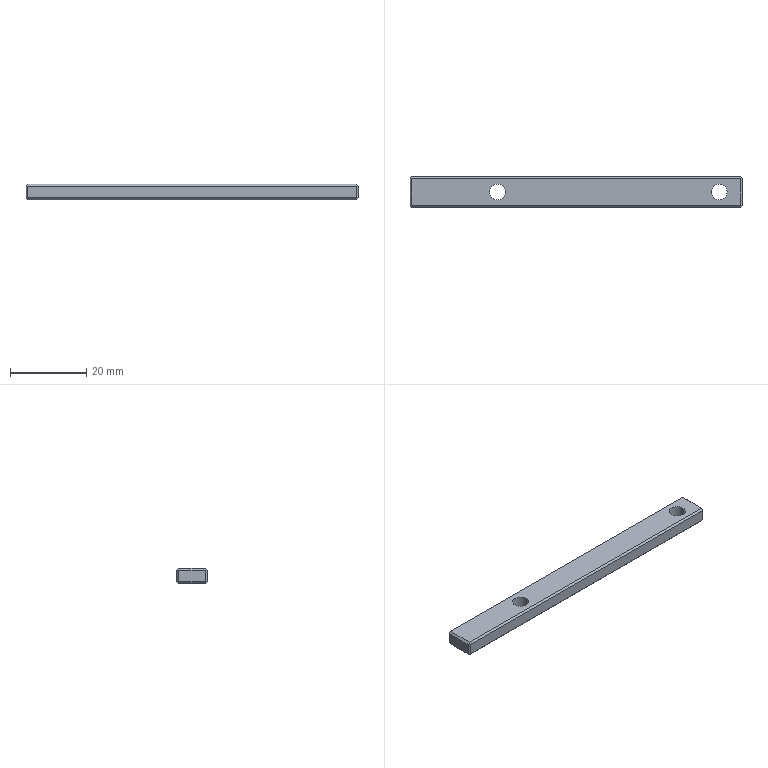Part | Creo | features DATUM PLANE 3, CHAMFER 1, COORDINATE SYSTEM 1, CURVE 1, PROTRUSION 1 | 1 solid | 22 faces | box 87 x 8 x 4 mm | volume 2624 mm3 | plane 18 | cylinder 4 | commonest cylinder face diameters 4.2 x4
STEP:
#1=CARTESIAN_POINT('',(0.,0.,0.));
#2=DIRECTION('',(0.,0.,1.));
#3=DIRECTION('',(1.,0.,0.));
#4=AXIS2_PLACEMENT_3D('',#1,#2,#3);
#5=CARTESIAN_POINT('',(43.,3.5,0.));
#6=VERTEX_POINT('',#5);
#7=CARTESIAN_POINT('',(43.,-3.5,0.));
#8=VERTEX_POINT('',#7);
#9=CARTESIAN_POINT('',(43.,3.5,0.));
#10=DIRECTION('',(0.,-1.,0.));
#11=VECTOR('',#10,7.);
#12=LINE('',#9,#11);
#13=EDGE_CURVE('',#6,#8,#12,.T.);
#14=ORIENTED_EDGE('',*,*,#13,.F.);
#15=CARTESIAN_POINT('',(-43.,3.5,0.));
#16=VERTEX_POINT('',#15);
#17=CARTESIAN_POINT('',(-43.,3.5,0.));
#18=DIRECTION('',(1.,0.,0.));
#19=VECTOR('',#18,86.);
#20=LINE('',#17,#19);
#21=EDGE_CURVE('',#16,#6,#20,.T.);
#22=ORIENTED_EDGE('',*,*,#21,.F.);
#23=CARTESIAN_POINT('',(-43.,-3.5,0.));
#24=VERTEX_POINT('',#23);
#25=CARTESIAN_POINT('',(-43.,-3.5,0.));
#26=DIRECTION('',(0.,1.,0.));
#27=VECTOR('',#26,7.);
#28=LINE('',#25,#27);
#29=EDGE_CURVE('',#24,#16,#28,.T.);
#30=ORIENTED_EDGE('',*,*,#29,.F.);
#31=CARTESIAN_POINT('',(43.,-3.5,0.));
#32=DIRECTION('',(-1.,0.,0.));
#33=VECTOR('',#32,86.);
#34=LINE('',#31,#33);
#35=EDGE_CURVE('',#8,#24,#34,.T.);
#36=ORIENTED_EDGE('',*,*,#35,.F.);
#37=EDGE_LOOP('',(#14,#22,#30,#36));
#38=FACE_OUTER_BOUND('',#37,.F.);
#39=CARTESIAN_POINT('',(-18.4,0.,0.));
#40=VERTEX_POINT('',#39);
#41=CARTESIAN_POINT('',(-22.6,0.,0.));
#42=VERTEX_POINT('',#41);
#43=CARTESIAN_POINT('',(-20.5,0.,0.));
#44=DIRECTION('',(0.,0.,-1.));
#45=DIRECTION('',(1.,0.,0.));
#46=AXIS2_PLACEMENT_3D('',#43,#44,#45);
#47=CIRCLE('',#46,2.1);
#48=EDGE_CURVE('',#40,#42,#47,.T.);
#49=ORIENTED_EDGE('',*,*,#48,.T.);
#50=CARTESIAN_POINT('',(-20.5,0.,0.));
#51=DIRECTION('',(0.,0.,-1.));
#52=DIRECTION('',(-1.,0.,0.));
#53=AXIS2_PLACEMENT_3D('',#50,#51,#52);
#54=CIRCLE('',#53,2.1);
#55=EDGE_CURVE('',#42,#40,#54,.T.);
#56=ORIENTED_EDGE('',*,*,#55,.T.);
#57=EDGE_LOOP('',(#49,#56));
#58=FACE_BOUND('',#57,.F.);
#59=CARTESIAN_POINT('',(39.6,0.,0.));
#60=VERTEX_POINT('',#59);
#61=CARTESIAN_POINT('',(35.4,0.,0.));
#62=VERTEX_POINT('',#61);
#63=CARTESIAN_POINT('',(37.5,0.,0.));
#64=DIRECTION('',(0.,0.,-1.));
#65=DIRECTION('',(1.,0.,0.));
#66=AXIS2_PLACEMENT_3D('',#63,#64,#65);
#67=CIRCLE('',#66,2.1);
#68=EDGE_CURVE('',#60,#62,#67,.T.);
#69=ORIENTED_EDGE('',*,*,#68,.T.);
#70=CARTESIAN_POINT('',(37.5,0.,0.));
#71=DIRECTION('',(0.,0.,-1.));
#72=DIRECTION('',(-1.,0.,0.));
#73=AXIS2_PLACEMENT_3D('',#70,#71,#72);
#74=CIRCLE('',#73,2.1);
#75=EDGE_CURVE('',#62,#60,#74,.T.);
#76=ORIENTED_EDGE('',*,*,#75,.T.);
#77=EDGE_LOOP('',(#69,#76));
#78=FACE_BOUND('',#77,.F.);
#79=CARTESIAN_POINT('',(0.,0.,0.));
#80=DIRECTION('',(0.,0.,1.));
#81=DIRECTION('',(1.,0.,0.));
#82=AXIS2_PLACEMENT_3D('',#79,#80,#81);
#83=PLANE('',#82);
#84=ADVANCED_FACE('',(#38,#58,#78),#83,.F.);
#85=ORIENTED_EDGE('',*,*,#68,.F.);
#86=CARTESIAN_POINT('',(39.6,0.,4.));
#87=VERTEX_POINT('',#86);
#88=CARTESIAN_POINT('',(39.6,0.,0.));
#89=DIRECTION('',(0.,0.,1.));
#90=VECTOR('',#89,4.);
#91=LINE('',#88,#90);
#92=EDGE_CURVE('',#60,#87,#91,.T.);
#93=ORIENTED_EDGE('',*,*,#92,.T.);
#94=CARTESIAN_POINT('',(35.4,0.,4.));
#95=VERTEX_POINT('',#94);
#96=CARTESIAN_POINT('',(37.5,0.,4.));
#97=DIRECTION('',(0.,0.,-1.));
#98=DIRECTION('',(1.,0.,0.));
#99=AXIS2_PLACEMENT_3D('',#96,#97,#98);
#100=CIRCLE('',#99,2.1);
#101=EDGE_CURVE('',#87,#95,#100,.T.);
#102=ORIENTED_EDGE('',*,*,#101,.T.);
#103=CARTESIAN_POINT('',(35.4,0.,0.));
#104=DIRECTION('',(0.,0.,1.));
#105=VECTOR('',#104,4.);
#106=LINE('',#103,#105);
#107=EDGE_CURVE('',#62,#95,#106,.T.);
#108=ORIENTED_EDGE('',*,*,#107,.F.);
#109=EDGE_LOOP('',(#85,#93,#102,#108));
#110=FACE_OUTER_BOUND('',#109,.F.);
#111=CARTESIAN_POINT('',(37.5,0.,0.));
#112=DIRECTION('',(0.,0.,1.));
#113=DIRECTION('',(1.,0.,0.));
#114=AXIS2_PLACEMENT_3D('',#111,#112,#113);
#115=CYLINDRICAL_SURFACE('',#114,2.1);
#116=ADVANCED_FACE('',(#110),#115,.F.);
#117=ORIENTED_EDGE('',*,*,#75,.F.);
#118=ORIENTED_EDGE('',*,*,#107,.T.);
#119=CARTESIAN_POINT('',(37.5,0.,4.));
#120=DIRECTION('',(0.,0.,-1.));
#121=DIRECTION('',(-1.,0.,0.));
#122=AXIS2_PLACEMENT_3D('',#119,#120,#121);
#123=CIRCLE('',#122,2.1);
#124=EDGE_CURVE('',#95,#87,#123,.T.);
#125=ORIENTED_EDGE('',*,*,#124,.T.);
#126=ORIENTED_EDGE('',*,*,#92,.F.);
#127=EDGE_LOOP('',(#117,#118,#125,#126));
#128=FACE_OUTER_BOUND('',#127,.F.);
#129=CARTESIAN_POINT('',(37.5,0.,0.));
#130=DIRECTION('',(0.,0.,1.));
#131=DIRECTION('',(1.,0.,0.));
#132=AXIS2_PLACEMENT_3D('',#129,#130,#131);
#133=CYLINDRICAL_SURFACE('',#132,2.1);
#134=ADVANCED_FACE('',(#128),#133,.F.);
#135=CARTESIAN_POINT('',(43.,-3.5,4.));
#136=VERTEX_POINT('',#135);
#137=CARTESIAN_POINT('',(43.,3.5,4.));
#138=VERTEX_POINT('',#137);
#139=CARTESIAN_POINT('',(43.,-3.5,4.));
#140=DIRECTION('',(0.,1.,0.));
#141=VECTOR('',#140,7.);
#142=LINE('',#139,#141);
#143=EDGE_CURVE('',#136,#138,#142,.T.);
#144=ORIENTED_EDGE('',*,*,#143,.F.);
#145=CARTESIAN_POINT('',(-43.,-3.5,4.));
#146=VERTEX_POINT('',#145);
#147=CARTESIAN_POINT('',(-43.,-3.5,4.));
#148=DIRECTION('',(1.,0.,0.));
#149=VECTOR('',#148,86.);
#150=LINE('',#147,#149);
#151=EDGE_CURVE('',#146,#136,#150,.T.);
#152=ORIENTED_EDGE('',*,*,#151,.F.);
#153=CARTESIAN_POINT('',(-43.,3.5,4.));
#154=VERTEX_POINT('',#153);
#155=CARTESIAN_POINT('',(-43.,3.5,4.));
#156=DIRECTION('',(0.,-1.,0.));
#157=VECTOR('',#156,7.);
#158=LINE('',#155,#157);
#159=EDGE_CURVE('',#154,#146,#158,.T.);
#160=ORIENTED_EDGE('',*,*,#159,.F.);
#161=CARTESIAN_POINT('',(43.,3.5,4.));
#162=DIRECTION('',(-1.,0.,0.));
#163=VECTOR('',#162,86.);
#164=LINE('',#161,#163);
#165=EDGE_CURVE('',#138,#154,#164,.T.);
#166=ORIENTED_EDGE('',*,*,#165,.F.);
#167=EDGE_LOOP('',(#144,#152,#160,#166));
#168=FACE_OUTER_BOUND('',#167,.F.);
#169=CARTESIAN_POINT('',(-18.4,0.,4.));
#170=VERTEX_POINT('',#169);
#171=CARTESIAN_POINT('',(-22.6,0.,4.));
#172=VERTEX_POINT('',#171);
#173=CARTESIAN_POINT('',(-20.5,0.,4.));
#174=DIRECTION('',(0.,0.,-1.));
#175=DIRECTION('',(1.,0.,0.));
#176=AXIS2_PLACEMENT_3D('',#173,#174,#175);
#177=CIRCLE('',#176,2.1);
#178=EDGE_CURVE('',#170,#172,#177,.T.);
#179=ORIENTED_EDGE('',*,*,#178,.F.);
#180=CARTESIAN_POINT('',(-20.5,0.,4.));
#181=DIRECTION('',(0.,0.,-1.));
#182=DIRECTION('',(-1.,0.,0.));
#183=AXIS2_PLACEMENT_3D('',#180,#181,#182);
#184=CIRCLE('',#183,2.1);
#185=EDGE_CURVE('',#172,#170,#184,.T.);
#186=ORIENTED_EDGE('',*,*,#185,.F.);
#187=EDGE_LOOP('',(#179,#186));
#188=FACE_BOUND('',#187,.F.);
#189=ORIENTED_EDGE('',*,*,#101,.F.);
#190=ORIENTED_EDGE('',*,*,#124,.F.);
#191=EDGE_LOOP('',(#189,#190));
#192=FACE_BOUND('',#191,.F.);
#193=CARTESIAN_POINT('',(0.,0.,4.));
#194=DIRECTION('',(0.,0.,1.));
#195=DIRECTION('',(1.,0.,0.));
#196=AXIS2_PLACEMENT_3D('',#193,#194,#195);
#197=PLANE('',#196);
#198=ADVANCED_FACE('',(#168,#188,#192),#197,.T.);
#199=ORIENTED_EDGE('',*,*,#48,.F.);
#200=CARTESIAN_POINT('',(-18.4,0.,0.));
#201=DIRECTION('',(0.,0.,1.));
#202=VECTOR('',#201,4.);
#203=LINE('',#200,#202);
#204=EDGE_CURVE('',#40,#170,#203,.T.);
#205=ORIENTED_EDGE('',*,*,#204,.T.);
#206=ORIENTED_EDGE('',*,*,#178,.T.);
#207=CARTESIAN_POINT('',(-22.6,0.,0.));
#208=DIRECTION('',(0.,0.,1.));
#209=VECTOR('',#208,4.);
#210=LINE('',#207,#209);
#211=EDGE_CURVE('',#42,#172,#210,.T.);
#212=ORIENTED_EDGE('',*,*,#211,.F.);
#213=EDGE_LOOP('',(#199,#205,#206,#212));
#214=FACE_OUTER_BOUND('',#213,.F.);
#215=CARTESIAN_POINT('',(-20.5,0.,0.));
#216=DIRECTION('',(0.,0.,1.));
#217=DIRECTION('',(1.,0.,0.));
#218=AXIS2_PLACEMENT_3D('',#215,#216,#217);
#219=CYLINDRICAL_SURFACE('',#218,2.1);
#220=ADVANCED_FACE('',(#214),#219,.F.);
#221=ORIENTED_EDGE('',*,*,#55,.F.);
#222=ORIENTED_EDGE('',*,*,#211,.T.);
#223=ORIENTED_EDGE('',*,*,#185,.T.);
#224=ORIENTED_EDGE('',*,*,#204,.F.);
#225=EDGE_LOOP('',(#221,#222,#223,#224));
#226=FACE_OUTER_BOUND('',#225,.F.);
#227=CARTESIAN_POINT('',(-20.5,0.,0.));
#228=DIRECTION('',(0.,0.,1.));
#229=DIRECTION('',(1.,0.,0.));
#230=AXIS2_PLACEMENT_3D('',#227,#228,#229);
#231=CYLINDRICAL_SURFACE('',#230,2.1);
#232=ADVANCED_FACE('',(#226),#231,.F.);
#233=CARTESIAN_POINT('',(43.5,-3.5,3.5));
#234=VERTEX_POINT('',#233);
#235=CARTESIAN_POINT('',(43.5,3.5,3.5));
#236=VERTEX_POINT('',#235);
#237=CARTESIAN_POINT('',(43.5,-3.5,3.5));
#238=DIRECTION('',(0.,1.,0.));
#239=VECTOR('',#238,7.);
#240=LINE('',#237,#239);
#241=EDGE_CURVE('',#234,#236,#240,.T.);
#242=ORIENTED_EDGE('',*,*,#241,.F.);
#243=CARTESIAN_POINT('',(43.25,-3.75,3.75));
#244=VERTEX_POINT('',#243);
#245=CARTESIAN_POINT('',(43.5,-3.5,3.5));
#246=DIRECTION('',(-0.5774,-0.5774,0.5774));
#247=VECTOR('',#246,0.433);
#248=LINE('',#245,#247);
#249=EDGE_CURVE('',#234,#244,#248,.T.);
#250=ORIENTED_EDGE('',*,*,#249,.T.);
#251=CARTESIAN_POINT('',(43.25,-3.75,3.75));
#252=DIRECTION('',(-0.5774,0.5774,0.5774));
#253=VECTOR('',#252,0.433);
#254=LINE('',#251,#253);
#255=EDGE_CURVE('',#244,#136,#254,.T.);
#256=ORIENTED_EDGE('',*,*,#255,.T.);
#257=ORIENTED_EDGE('',*,*,#143,.T.);
#258=CARTESIAN_POINT('',(43.25,3.75,3.75));
#259=VERTEX_POINT('',#258);
#260=CARTESIAN_POINT('',(43.,3.5,4.));
#261=DIRECTION('',(0.5774,0.5774,-0.5774));
#262=VECTOR('',#261,0.433);
#263=LINE('',#260,#262);
#264=EDGE_CURVE('',#138,#259,#263,.T.);
#265=ORIENTED_EDGE('',*,*,#264,.T.);
#266=CARTESIAN_POINT('',(43.25,3.75,3.75));
#267=DIRECTION('',(0.5774,-0.5774,-0.5774));
#268=VECTOR('',#267,0.433);
#269=LINE('',#266,#268);
#270=EDGE_CURVE('',#259,#236,#269,.T.);
#271=ORIENTED_EDGE('',*,*,#270,.T.);
#272=EDGE_LOOP('',(#242,#250,#256,#257,#265,#271));
#273=FACE_OUTER_BOUND('',#272,.F.);
#274=CARTESIAN_POINT('',(43.25,0.,3.75));
#275=DIRECTION('',(0.7071,0.,0.7071));
#276=DIRECTION('',(0.7071,0.,-0.7071));
#277=AXIS2_PLACEMENT_3D('',#274,#275,#276);
#278=PLANE('',#277);
#279=ADVANCED_FACE('',(#273),#278,.T.);
#280=CARTESIAN_POINT('',(43.5,3.5,0.5));
#281=VERTEX_POINT('',#280);
#282=CARTESIAN_POINT('',(43.5,-3.5,0.5));
#283=VERTEX_POINT('',#282);
#284=CARTESIAN_POINT('',(43.5,3.5,0.5));
#285=DIRECTION('',(0.,-1.,0.));
#286=VECTOR('',#285,7.);
#287=LINE('',#284,#286);
#288=EDGE_CURVE('',#281,#283,#287,.T.);
#289=ORIENTED_EDGE('',*,*,#288,.T.);
#290=CARTESIAN_POINT('',(43.5,-3.5,3.5));
#291=DIRECTION('',(0.,0.,-1.));
#292=VECTOR('',#291,3.);
#293=LINE('',#290,#292);
#294=EDGE_CURVE('',#234,#283,#293,.T.);
#295=ORIENTED_EDGE('',*,*,#294,.F.);
#296=ORIENTED_EDGE('',*,*,#241,.T.);
#297=CARTESIAN_POINT('',(43.5,3.5,3.5));
#298=DIRECTION('',(0.,0.,-1.));
#299=VECTOR('',#298,3.);
#300=LINE('',#297,#299);
#301=EDGE_CURVE('',#236,#281,#300,.T.);
#302=ORIENTED_EDGE('',*,*,#301,.T.);
#303=EDGE_LOOP('',(#289,#295,#296,#302));
#304=FACE_OUTER_BOUND('',#303,.F.);
#305=CARTESIAN_POINT('',(43.5,-4.,0.));
#306=DIRECTION('',(1.,0.,0.));
#307=DIRECTION('',(0.,1.,0.));
#308=AXIS2_PLACEMENT_3D('',#305,#306,#307);
#309=PLANE('',#308);
#310=ADVANCED_FACE('',(#304),#309,.T.);
#311=ORIENTED_EDGE('',*,*,#288,.F.);
#312=CARTESIAN_POINT('',(43.25,3.75,0.25));
#313=VERTEX_POINT('',#312);
#314=CARTESIAN_POINT('',(43.5,3.5,0.5));
#315=DIRECTION('',(-0.5774,0.5774,-0.5774));
#316=VECTOR('',#315,0.433);
#317=LINE('',#314,#316);
#318=EDGE_CURVE('',#281,#313,#317,.T.);
#319=ORIENTED_EDGE('',*,*,#318,.T.);
#320=CARTESIAN_POINT('',(43.25,3.75,0.25));
#321=DIRECTION('',(-0.5774,-0.5774,-0.5774));
#322=VECTOR('',#321,0.433);
#323=LINE('',#320,#322);
#324=EDGE_CURVE('',#313,#6,#323,.T.);
#325=ORIENTED_EDGE('',*,*,#324,.T.);
#326=ORIENTED_EDGE('',*,*,#13,.T.);
#327=CARTESIAN_POINT('',(43.25,-3.75,0.25));
#328=VERTEX_POINT('',#327);
#329=CARTESIAN_POINT('',(43.,-3.5,0.));
#330=DIRECTION('',(0.5774,-0.5774,0.5774));
#331=VECTOR('',#330,0.433);
#332=LINE('',#329,#331);
#333=EDGE_CURVE('',#8,#328,#332,.T.);
#334=ORIENTED_EDGE('',*,*,#333,.T.);
#335=CARTESIAN_POINT('',(43.25,-3.75,0.25));
#336=DIRECTION('',(0.5774,0.5774,0.5774));
#337=VECTOR('',#336,0.433);
#338=LINE('',#335,#337);
#339=EDGE_CURVE('',#328,#283,#338,.T.);
#340=ORIENTED_EDGE('',*,*,#339,.T.);
#341=EDGE_LOOP('',(#311,#319,#325,#326,#334,#340));
#342=FACE_OUTER_BOUND('',#341,.F.);
#343=CARTESIAN_POINT('',(43.25,0.,0.25));
#344=DIRECTION('',(0.7071,0.,-0.7071));
#345=DIRECTION('',(0.7071,0.,0.7071));
#346=AXIS2_PLACEMENT_3D('',#343,#344,#345);
#347=PLANE('',#346);
#348=ADVANCED_FACE('',(#342),#347,.T.);
#349=CARTESIAN_POINT('',(43.,4.,3.5));
#350=VERTEX_POINT('',#349);
#351=CARTESIAN_POINT('',(43.,4.,0.5));
#352=VERTEX_POINT('',#351);
#353=CARTESIAN_POINT('',(43.,4.,3.5));
#354=DIRECTION('',(0.,0.,-1.));
#355=VECTOR('',#354,3.);
#356=LINE('',#353,#355);
#357=EDGE_CURVE('',#350,#352,#356,.T.);
#358=ORIENTED_EDGE('',*,*,#357,.T.);
#359=CARTESIAN_POINT('',(43.,4.,0.5));
#360=DIRECTION('',(0.5774,-0.5774,-0.5774));
#361=VECTOR('',#360,0.433);
#362=LINE('',#359,#361);
#363=EDGE_CURVE('',#352,#313,#362,.T.);
#364=ORIENTED_EDGE('',*,*,#363,.T.);
#365=ORIENTED_EDGE('',*,*,#318,.F.);
#366=ORIENTED_EDGE('',*,*,#301,.F.);
#367=ORIENTED_EDGE('',*,*,#270,.F.);
#368=CARTESIAN_POINT('',(43.,4.,3.5));
#369=DIRECTION('',(0.5774,-0.5774,0.5774));
#370=VECTOR('',#369,0.433);
#371=LINE('',#368,#370);
#372=EDGE_CURVE('',#350,#259,#371,.T.);
#373=ORIENTED_EDGE('',*,*,#372,.F.);
#374=EDGE_LOOP('',(#358,#364,#365,#366,#367,#373));
#375=FACE_OUTER_BOUND('',#374,.F.);
#376=CARTESIAN_POINT('',(43.25,3.75,2.));
#377=DIRECTION('',(0.7071,0.7071,0.));
#378=DIRECTION('',(0.7071,-0.7071,0.));
#379=AXIS2_PLACEMENT_3D('',#376,#377,#378);
#380=PLANE('',#379);
#381=ADVANCED_FACE('',(#375),#380,.T.);
#382=CARTESIAN_POINT('',(-43.,4.,3.5));
#383=VERTEX_POINT('',#382);
#384=CARTESIAN_POINT('',(43.,4.,3.5));
#385=DIRECTION('',(-1.,0.,0.));
#386=VECTOR('',#385,86.);
#387=LINE('',#384,#386);
#388=EDGE_CURVE('',#350,#383,#387,.T.);
#389=ORIENTED_EDGE('',*,*,#388,.T.);
#390=CARTESIAN_POINT('',(-43.,4.,0.5));
#391=VERTEX_POINT('',#390);
#392=CARTESIAN_POINT('',(-43.,4.,3.5));
#393=DIRECTION('',(0.,0.,-1.));
#394=VECTOR('',#393,3.);
#395=LINE('',#392,#394);
#396=EDGE_CURVE('',#383,#391,#395,.T.);
#397=ORIENTED_EDGE('',*,*,#396,.T.);
#398=CARTESIAN_POINT('',(-43.,4.,0.5));
#399=DIRECTION('',(1.,0.,0.));
#400=VECTOR('',#399,86.);
#401=LINE('',#398,#400);
#402=EDGE_CURVE('',#391,#352,#401,.T.);
#403=ORIENTED_EDGE('',*,*,#402,.T.);
#404=ORIENTED_EDGE('',*,*,#357,.F.);
#405=EDGE_LOOP('',(#389,#397,#403,#404));
#406=FACE_OUTER_BOUND('',#405,.F.);
#407=CARTESIAN_POINT('',(43.5,4.,0.));
#408=DIRECTION('',(0.,1.,0.));
#409=DIRECTION('',(-1.,0.,0.));
#410=AXIS2_PLACEMENT_3D('',#407,#408,#409);
#411=PLANE('',#410);
#412=ADVANCED_FACE('',(#406),#411,.T.);
#413=ORIENTED_EDGE('',*,*,#388,.F.);
#414=ORIENTED_EDGE('',*,*,#372,.T.);
#415=ORIENTED_EDGE('',*,*,#264,.F.);
#416=ORIENTED_EDGE('',*,*,#165,.T.);
#417=CARTESIAN_POINT('',(-43.25,3.75,3.75));
#418=VERTEX_POINT('',#417);
#419=CARTESIAN_POINT('',(-43.,3.5,4.));
#420=DIRECTION('',(-0.5774,0.5774,-0.5774));
#421=VECTOR('',#420,0.433);
#422=LINE('',#419,#421);
#423=EDGE_CURVE('',#154,#418,#422,.T.);
#424=ORIENTED_EDGE('',*,*,#423,.T.);
#425=CARTESIAN_POINT('',(-43.25,3.75,3.75));
#426=DIRECTION('',(0.5774,0.5774,-0.5774));
#427=VECTOR('',#426,0.433);
#428=LINE('',#425,#427);
#429=EDGE_CURVE('',#418,#383,#428,.T.);
#430=ORIENTED_EDGE('',*,*,#429,.T.);
#431=EDGE_LOOP('',(#413,#414,#415,#416,#424,#430));
#432=FACE_OUTER_BOUND('',#431,.F.);
#433=CARTESIAN_POINT('',(0.,3.75,3.75));
#434=DIRECTION('',(0.,0.7071,0.7071));
#435=DIRECTION('',(0.,0.7071,-0.7071));
#436=AXIS2_PLACEMENT_3D('',#433,#434,#435);
#437=PLANE('',#436);
#438=ADVANCED_FACE('',(#432),#437,.T.);
#439=CARTESIAN_POINT('',(-43.5,3.5,3.5));
#440=VERTEX_POINT('',#439);
#441=CARTESIAN_POINT('',(-43.5,-3.5,3.5));
#442=VERTEX_POINT('',#441);
#443=CARTESIAN_POINT('',(-43.5,3.5,3.5));
#444=DIRECTION('',(0.,-1.,0.));
#445=VECTOR('',#444,7.);
#446=LINE('',#443,#445);
#447=EDGE_CURVE('',#440,#442,#446,.T.);
#448=ORIENTED_EDGE('',*,*,#447,.F.);
#449=CARTESIAN_POINT('',(-43.5,3.5,3.5));
#450=DIRECTION('',(0.5774,0.5774,0.5774));
#451=VECTOR('',#450,0.433);
#452=LINE('',#449,#451);
#453=EDGE_CURVE('',#440,#418,#452,.T.);
#454=ORIENTED_EDGE('',*,*,#453,.T.);
#455=ORIENTED_EDGE('',*,*,#423,.F.);
#456=ORIENTED_EDGE('',*,*,#159,.T.);
#457=CARTESIAN_POINT('',(-43.25,-3.75,3.75));
#458=VERTEX_POINT('',#457);
#459=CARTESIAN_POINT('',(-43.,-3.5,4.));
#460=DIRECTION('',(-0.5774,-0.5774,-0.5774));
#461=VECTOR('',#460,0.433);
#462=LINE('',#459,#461);
#463=EDGE_CURVE('',#146,#458,#462,.T.);
#464=ORIENTED_EDGE('',*,*,#463,.T.);
#465=CARTESIAN_POINT('',(-43.25,-3.75,3.75));
#466=DIRECTION('',(-0.5774,0.5774,-0.5774));
#467=VECTOR('',#466,0.433);
#468=LINE('',#465,#467);
#469=EDGE_CURVE('',#458,#442,#468,.T.);
#470=ORIENTED_EDGE('',*,*,#469,.T.);
#471=EDGE_LOOP('',(#448,#454,#455,#456,#464,#470));
#472=FACE_OUTER_BOUND('',#471,.F.);
#473=CARTESIAN_POINT('',(-43.25,0.,3.75));
#474=DIRECTION('',(-0.7071,0.,0.7071));
#475=DIRECTION('',(-0.7071,0.,-0.7071));
#476=AXIS2_PLACEMENT_3D('',#473,#474,#475);
#477=PLANE('',#476);
#478=ADVANCED_FACE('',(#472),#477,.T.);
#479=CARTESIAN_POINT('',(-43.5,-3.5,0.5));
#480=VERTEX_POINT('',#479);
#481=CARTESIAN_POINT('',(-43.5,3.5,0.5));
#482=VERTEX_POINT('',#481);
#483=CARTESIAN_POINT('',(-43.5,-3.5,0.5));
#484=DIRECTION('',(0.,1.,0.));
#485=VECTOR('',#484,7.);
#486=LINE('',#483,#485);
#487=EDGE_CURVE('',#480,#482,#486,.T.);
#488=ORIENTED_EDGE('',*,*,#487,.T.);
#489=CARTESIAN_POINT('',(-43.5,3.5,3.5));
#490=DIRECTION('',(0.,0.,-1.));
#491=VECTOR('',#490,3.);
#492=LINE('',#489,#491);
#493=EDGE_CURVE('',#440,#482,#492,.T.);
#494=ORIENTED_EDGE('',*,*,#493,.F.);
#495=ORIENTED_EDGE('',*,*,#447,.T.);
#496=CARTESIAN_POINT('',(-43.5,-3.5,3.5));
#497=DIRECTION('',(0.,0.,-1.));
#498=VECTOR('',#497,3.);
#499=LINE('',#496,#498);
#500=EDGE_CURVE('',#442,#480,#499,.T.);
#501=ORIENTED_EDGE('',*,*,#500,.T.);
#502=EDGE_LOOP('',(#488,#494,#495,#501));
#503=FACE_OUTER_BOUND('',#502,.F.);
#504=CARTESIAN_POINT('',(-43.5,4.,0.));
#505=DIRECTION('',(-1.,0.,0.));
#506=DIRECTION('',(0.,-1.,0.));
#507=AXIS2_PLACEMENT_3D('',#504,#505,#506);
#508=PLANE('',#507);
#509=ADVANCED_FACE('',(#503),#508,.T.);
#510=ORIENTED_EDGE('',*,*,#29,.T.);
#511=CARTESIAN_POINT('',(-43.25,3.75,0.25));
#512=VERTEX_POINT('',#511);
#513=CARTESIAN_POINT('',(-43.25,3.75,0.25));
#514=DIRECTION('',(0.5774,-0.5774,-0.5774));
#515=VECTOR('',#514,0.433);
#516=LINE('',#513,#515);
#517=EDGE_CURVE('',#512,#16,#516,.T.);
#518=ORIENTED_EDGE('',*,*,#517,.F.);
#519=CARTESIAN_POINT('',(-43.5,3.5,0.5));
#520=DIRECTION('',(0.5774,0.5774,-0.5774));
#521=VECTOR('',#520,0.433);
#522=LINE('',#519,#521);
#523=EDGE_CURVE('',#482,#512,#522,.T.);
#524=ORIENTED_EDGE('',*,*,#523,.F.);
#525=ORIENTED_EDGE('',*,*,#487,.F.);
#526=CARTESIAN_POINT('',(-43.25,-3.75,0.25));
#527=VERTEX_POINT('',#526);
#528=CARTESIAN_POINT('',(-43.5,-3.5,0.5));
#529=DIRECTION('',(0.5774,-0.5774,-0.5774));
#530=VECTOR('',#529,0.433);
#531=LINE('',#528,#530);
#532=EDGE_CURVE('',#480,#527,#531,.T.);
#533=ORIENTED_EDGE('',*,*,#532,.T.);
#534=CARTESIAN_POINT('',(-43.25,-3.75,0.25));
#535=DIRECTION('',(0.5774,0.5774,-0.5774));
#536=VECTOR('',#535,0.433);
#537=LINE('',#534,#536);
#538=EDGE_CURVE('',#527,#24,#537,.T.);
#539=ORIENTED_EDGE('',*,*,#538,.T.);
#540=EDGE_LOOP('',(#510,#518,#524,#525,#533,#539));
#541=FACE_OUTER_BOUND('',#540,.F.);
#542=CARTESIAN_POINT('',(-43.25,0.,0.25));
#543=DIRECTION('',(-0.7071,0.,-0.7071));
#544=DIRECTION('',(-0.7071,0.,0.7071));
#545=AXIS2_PLACEMENT_3D('',#542,#543,#544);
#546=PLANE('',#545);
#547=ADVANCED_FACE('',(#541),#546,.T.);
#548=ORIENTED_EDGE('',*,*,#21,.T.);
#549=ORIENTED_EDGE('',*,*,#324,.F.);
#550=ORIENTED_EDGE('',*,*,#363,.F.);
#551=ORIENTED_EDGE('',*,*,#402,.F.);
#552=CARTESIAN_POINT('',(-43.,4.,0.5));
#553=DIRECTION('',(-0.5774,-0.5774,-0.5774));
#554=VECTOR('',#553,0.433);
#555=LINE('',#552,#554);
#556=EDGE_CURVE('',#391,#512,#555,.T.);
#557=ORIENTED_EDGE('',*,*,#556,.T.);
#558=ORIENTED_EDGE('',*,*,#517,.T.);
#559=EDGE_LOOP('',(#548,#549,#550,#551,#557,#558));
#560=FACE_OUTER_BOUND('',#559,.F.);
#561=CARTESIAN_POINT('',(0.,3.75,0.25));
#562=DIRECTION('',(0.,0.7071,-0.7071));
#563=DIRECTION('',(0.,0.7071,0.7071));
#564=AXIS2_PLACEMENT_3D('',#561,#562,#563);
#565=PLANE('',#564);
#566=ADVANCED_FACE('',(#560),#565,.T.);
#567=ORIENTED_EDGE('',*,*,#493,.T.);
#568=ORIENTED_EDGE('',*,*,#523,.T.);
#569=ORIENTED_EDGE('',*,*,#556,.F.);
#570=ORIENTED_EDGE('',*,*,#396,.F.);
#571=ORIENTED_EDGE('',*,*,#429,.F.);
#572=ORIENTED_EDGE('',*,*,#453,.F.);
#573=EDGE_LOOP('',(#567,#568,#569,#570,#571,#572));
#574=FACE_OUTER_BOUND('',#573,.F.);
#575=CARTESIAN_POINT('',(-43.25,3.75,2.));
#576=DIRECTION('',(-0.7071,0.7071,0.));
#577=DIRECTION('',(0.7071,0.7071,0.));
#578=AXIS2_PLACEMENT_3D('',#575,#576,#577);
#579=PLANE('',#578);
#580=ADVANCED_FACE('',(#574),#579,.T.);
#581=CARTESIAN_POINT('',(-43.,-4.,3.5));
#582=VERTEX_POINT('',#581);
#583=CARTESIAN_POINT('',(-43.,-4.,0.5));
#584=VERTEX_POINT('',#583);
#585=CARTESIAN_POINT('',(-43.,-4.,3.5));
#586=DIRECTION('',(0.,0.,-1.));
#587=VECTOR('',#586,3.);
#588=LINE('',#585,#587);
#589=EDGE_CURVE('',#582,#584,#588,.T.);
#590=ORIENTED_EDGE('',*,*,#589,.T.);
#591=CARTESIAN_POINT('',(-43.,-4.,0.5));
#592=DIRECTION('',(-0.5774,0.5774,-0.5774));
#593=VECTOR('',#592,0.433);
#594=LINE('',#591,#593);
#595=EDGE_CURVE('',#584,#527,#594,.T.);
#596=ORIENTED_EDGE('',*,*,#595,.T.);
#597=ORIENTED_EDGE('',*,*,#532,.F.);
#598=ORIENTED_EDGE('',*,*,#500,.F.);
#599=ORIENTED_EDGE('',*,*,#469,.F.);
#600=CARTESIAN_POINT('',(-43.,-4.,3.5));
#601=DIRECTION('',(-0.5774,0.5774,0.5774));
#602=VECTOR('',#601,0.433);
#603=LINE('',#600,#602);
#604=EDGE_CURVE('',#582,#458,#603,.T.);
#605=ORIENTED_EDGE('',*,*,#604,.F.);
#606=EDGE_LOOP('',(#590,#596,#597,#598,#599,#605));
#607=FACE_OUTER_BOUND('',#606,.F.);
#608=CARTESIAN_POINT('',(-43.25,-3.75,2.));
#609=DIRECTION('',(-0.7071,-0.7071,0.));
#610=DIRECTION('',(-0.7071,0.7071,0.));
#611=AXIS2_PLACEMENT_3D('',#608,#609,#610);
#612=PLANE('',#611);
#613=ADVANCED_FACE('',(#607),#612,.T.);
#614=ORIENTED_EDGE('',*,*,#589,.F.);
#615=CARTESIAN_POINT('',(43.,-4.,3.5));
#616=VERTEX_POINT('',#615);
#617=CARTESIAN_POINT('',(-43.,-4.,3.5));
#618=DIRECTION('',(1.,0.,0.));
#619=VECTOR('',#618,86.);
#620=LINE('',#617,#619);
#621=EDGE_CURVE('',#582,#616,#620,.T.);
#622=ORIENTED_EDGE('',*,*,#621,.T.);
#623=CARTESIAN_POINT('',(43.,-4.,0.5));
#624=VERTEX_POINT('',#623);
#625=CARTESIAN_POINT('',(43.,-4.,3.5));
#626=DIRECTION('',(0.,0.,-1.));
#627=VECTOR('',#626,3.);
#628=LINE('',#625,#627);
#629=EDGE_CURVE('',#616,#624,#628,.T.);
#630=ORIENTED_EDGE('',*,*,#629,.T.);
#631=CARTESIAN_POINT('',(43.,-4.,0.5));
#632=DIRECTION('',(-1.,0.,0.));
#633=VECTOR('',#632,86.);
#634=LINE('',#631,#633);
#635=EDGE_CURVE('',#624,#584,#634,.T.);
#636=ORIENTED_EDGE('',*,*,#635,.T.);
#637=EDGE_LOOP('',(#614,#622,#630,#636));
#638=FACE_OUTER_BOUND('',#637,.F.);
#639=CARTESIAN_POINT('',(-43.5,-4.,0.));
#640=DIRECTION('',(0.,-1.,0.));
#641=DIRECTION('',(1.,0.,0.));
#642=AXIS2_PLACEMENT_3D('',#639,#640,#641);
#643=PLANE('',#642);
#644=ADVANCED_FACE('',(#638),#643,.T.);
#645=ORIENTED_EDGE('',*,*,#151,.T.);
#646=ORIENTED_EDGE('',*,*,#255,.F.);
#647=CARTESIAN_POINT('',(43.,-4.,3.5));
#648=DIRECTION('',(0.5774,0.5774,0.5774));
#649=VECTOR('',#648,0.433);
#650=LINE('',#647,#649);
#651=EDGE_CURVE('',#616,#244,#650,.T.);
#652=ORIENTED_EDGE('',*,*,#651,.F.);
#653=ORIENTED_EDGE('',*,*,#621,.F.);
#654=ORIENTED_EDGE('',*,*,#604,.T.);
#655=ORIENTED_EDGE('',*,*,#463,.F.);
#656=EDGE_LOOP('',(#645,#646,#652,#653,#654,#655));
#657=FACE_OUTER_BOUND('',#656,.F.);
#658=CARTESIAN_POINT('',(0.,-3.75,3.75));
#659=DIRECTION('',(0.,-0.7071,0.7071));
#660=DIRECTION('',(0.,-0.7071,-0.7071));
#661=AXIS2_PLACEMENT_3D('',#658,#659,#660);
#662=PLANE('',#661);
#663=ADVANCED_FACE('',(#657),#662,.T.);
#664=ORIENTED_EDGE('',*,*,#294,.T.);
#665=ORIENTED_EDGE('',*,*,#339,.F.);
#666=CARTESIAN_POINT('',(43.,-4.,0.5));
#667=DIRECTION('',(0.5774,0.5774,-0.5774));
#668=VECTOR('',#667,0.433);
#669=LINE('',#666,#668);
#670=EDGE_CURVE('',#624,#328,#669,.T.);
#671=ORIENTED_EDGE('',*,*,#670,.F.);
#672=ORIENTED_EDGE('',*,*,#629,.F.);
#673=ORIENTED_EDGE('',*,*,#651,.T.);
#674=ORIENTED_EDGE('',*,*,#249,.F.);
#675=EDGE_LOOP('',(#664,#665,#671,#672,#673,#674));
#676=FACE_OUTER_BOUND('',#675,.F.);
#677=CARTESIAN_POINT('',(43.25,-3.75,2.));
#678=DIRECTION('',(0.7071,-0.7071,0.));
#679=DIRECTION('',(-0.7071,-0.7071,0.));
#680=AXIS2_PLACEMENT_3D('',#677,#678,#679);
#681=PLANE('',#680);
#682=ADVANCED_FACE('',(#676),#681,.T.);
#683=ORIENTED_EDGE('',*,*,#635,.F.);
#684=ORIENTED_EDGE('',*,*,#670,.T.);
#685=ORIENTED_EDGE('',*,*,#333,.F.);
#686=ORIENTED_EDGE('',*,*,#35,.T.);
#687=ORIENTED_EDGE('',*,*,#538,.F.);
#688=ORIENTED_EDGE('',*,*,#595,.F.);
#689=EDGE_LOOP('',(#683,#684,#685,#686,#687,#688));
#690=FACE_OUTER_BOUND('',#689,.F.);
#691=CARTESIAN_POINT('',(0.,-3.75,0.25));
#692=DIRECTION('',(0.,-0.7071,-0.7071));
#693=DIRECTION('',(0.,-0.7071,0.7071));
#694=AXIS2_PLACEMENT_3D('',#691,#692,#693);
#695=PLANE('',#694);
#696=ADVANCED_FACE('',(#690),#695,.T.);
#697=CLOSED_SHELL('',(#84,#116,#134,#198,#220,#232,#279,#310,#348,#381,#412,#438,#478,#509,#547,#566,#580,#613,#644,#663,#682,#696));
#698=MANIFOLD_SOLID_BREP('',#697);
#699=(LENGTH_UNIT()NAMED_UNIT(*)SI_UNIT(.MILLI.,.METRE.));
#700=UNCERTAINTY_MEASURE_WITH_UNIT(LENGTH_MEASURE(0.008746),#699,'','');
#701=(NAMED_UNIT(*)PLANE_ANGLE_UNIT()SI_UNIT($,.RADIAN.));
#702=PLANE_ANGLE_MEASURE_WITH_UNIT(PLANE_ANGLE_MEASURE(0.01745),#701);
#703=(CONVERSION_BASED_UNIT('DEGREE',#702)NAMED_UNIT(*)PLANE_ANGLE_UNIT());
#704=(NAMED_UNIT(*)SI_UNIT($,.STERADIAN.)SOLID_ANGLE_UNIT());
#705=(GEOMETRIC_REPRESENTATION_CONTEXT(3)GLOBAL_UNCERTAINTY_ASSIGNED_CONTEXT((#700))GLOBAL_UNIT_ASSIGNED_CONTEXT((#699,#703,#704))REPRESENTATION_CONTEXT('',''));
#706=ADVANCED_BREP_SHAPE_REPRESENTATION('',(#4,#698),#705);